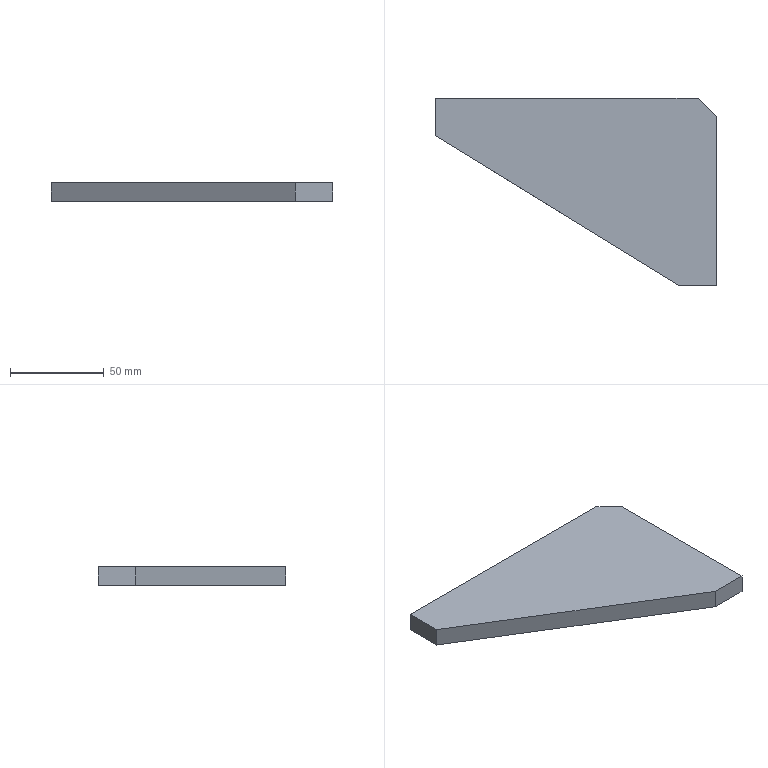Part | SolidWorks | features Chamfer 1, Extrusion 1 | 1 solid | 8 faces | box 150 x 100 x 10 mm | volume 97500 mm3 | plane 8
STEP:
#1=CARTESIAN_POINT('',(-150.,0.,0.));
#2=VERTEX_POINT('',#1);
#3=CARTESIAN_POINT('',(-150.,-20.,0.));
#4=VERTEX_POINT('',#3);
#5=CARTESIAN_POINT('',(-150.,0.,0.));
#6=DIRECTION('',(0.,-1.,0.));
#7=VECTOR('',#6,1000.);
#8=LINE('',#5,#7);
#9=EDGE_CURVE('',#2,#4,#8,.T.);
#10=ORIENTED_EDGE('',*,*,#9,.F.);
#11=CARTESIAN_POINT('',(-150.,0.,-10.));
#12=VERTEX_POINT('',#11);
#13=CARTESIAN_POINT('',(-150.,0.,-10.));
#14=DIRECTION('',(0.,0.,1.));
#15=VECTOR('',#14,1000.);
#16=LINE('',#13,#15);
#17=EDGE_CURVE('',#12,#2,#16,.T.);
#18=ORIENTED_EDGE('',*,*,#17,.F.);
#19=CARTESIAN_POINT('',(-150.,-20.,-10.));
#20=VERTEX_POINT('',#19);
#21=CARTESIAN_POINT('',(-150.,0.,-10.));
#22=DIRECTION('',(0.,-1.,0.));
#23=VECTOR('',#22,1000.);
#24=LINE('',#21,#23);
#25=EDGE_CURVE('',#12,#20,#24,.T.);
#26=ORIENTED_EDGE('',*,*,#25,.T.);
#27=CARTESIAN_POINT('',(-150.,-20.,-10.));
#28=DIRECTION('',(0.,0.,1.));
#29=VECTOR('',#28,1000.);
#30=LINE('',#27,#29);
#31=EDGE_CURVE('',#20,#4,#30,.T.);
#32=ORIENTED_EDGE('',*,*,#31,.T.);
#33=EDGE_LOOP('',(#10,#18,#26,#32));
#34=FACE_OUTER_BOUND('',#33,.T.);
#35=CARTESIAN_POINT('',(-150.,0.,-10.));
#36=DIRECTION('',(-1.,0.,0.));
#37=DIRECTION('',(0.,0.,1.));
#38=AXIS2_PLACEMENT_3D('',#35,#36,#37);
#39=PLANE('',#38);
#40=ADVANCED_FACE('',(#34),#39,.T.);
#41=CARTESIAN_POINT('',(-10.,0.,0.));
#42=VERTEX_POINT('',#41);
#43=CARTESIAN_POINT('',(0.,0.,0.));
#44=DIRECTION('',(-1.,0.,0.));
#45=VECTOR('',#44,1000.);
#46=LINE('',#43,#45);
#47=EDGE_CURVE('',#42,#2,#46,.T.);
#48=ORIENTED_EDGE('',*,*,#47,.F.);
#49=CARTESIAN_POINT('',(-10.,0.,-10.));
#50=VERTEX_POINT('',#49);
#51=CARTESIAN_POINT('',(-10.,0.,-10.));
#52=DIRECTION('',(0.,0.,-1.));
#53=VECTOR('',#52,1000.);
#54=LINE('',#51,#53);
#55=EDGE_CURVE('',#42,#50,#54,.T.);
#56=ORIENTED_EDGE('',*,*,#55,.T.);
#57=CARTESIAN_POINT('',(0.,0.,-10.));
#58=DIRECTION('',(-1.,0.,0.));
#59=VECTOR('',#58,1000.);
#60=LINE('',#57,#59);
#61=EDGE_CURVE('',#50,#12,#60,.T.);
#62=ORIENTED_EDGE('',*,*,#61,.T.);
#63=ORIENTED_EDGE('',*,*,#17,.T.);
#64=EDGE_LOOP('',(#48,#56,#62,#63));
#65=FACE_OUTER_BOUND('',#64,.T.);
#66=CARTESIAN_POINT('',(0.,0.,-10.));
#67=DIRECTION('',(0.,1.,0.));
#68=DIRECTION('',(-1.,0.,0.));
#69=AXIS2_PLACEMENT_3D('',#66,#67,#68);
#70=PLANE('',#69);
#71=ADVANCED_FACE('',(#65),#70,.T.);
#72=CARTESIAN_POINT('',(0.,-100.,-10.));
#73=VERTEX_POINT('',#72);
#74=CARTESIAN_POINT('',(0.,-10.,-10.));
#75=VERTEX_POINT('',#74);
#76=CARTESIAN_POINT('',(0.,-100.,-10.));
#77=DIRECTION('',(0.,1.,0.));
#78=VECTOR('',#77,1000.);
#79=LINE('',#76,#78);
#80=EDGE_CURVE('',#73,#75,#79,.T.);
#81=ORIENTED_EDGE('',*,*,#80,.T.);
#82=CARTESIAN_POINT('',(0.,-10.,0.));
#83=VERTEX_POINT('',#82);
#84=CARTESIAN_POINT('',(0.,-10.,-10.));
#85=DIRECTION('',(0.,0.,1.));
#86=VECTOR('',#85,1000.);
#87=LINE('',#84,#86);
#88=EDGE_CURVE('',#75,#83,#87,.T.);
#89=ORIENTED_EDGE('',*,*,#88,.T.);
#90=CARTESIAN_POINT('',(0.,-100.,0.));
#91=VERTEX_POINT('',#90);
#92=CARTESIAN_POINT('',(0.,-100.,0.));
#93=DIRECTION('',(0.,1.,0.));
#94=VECTOR('',#93,1000.);
#95=LINE('',#92,#94);
#96=EDGE_CURVE('',#91,#83,#95,.T.);
#97=ORIENTED_EDGE('',*,*,#96,.F.);
#98=CARTESIAN_POINT('',(0.,-100.,-10.));
#99=DIRECTION('',(0.,0.,1.));
#100=VECTOR('',#99,1000.);
#101=LINE('',#98,#100);
#102=EDGE_CURVE('',#73,#91,#101,.T.);
#103=ORIENTED_EDGE('',*,*,#102,.F.);
#104=EDGE_LOOP('',(#81,#89,#97,#103));
#105=FACE_OUTER_BOUND('',#104,.T.);
#106=CARTESIAN_POINT('',(0.,-100.,-10.));
#107=DIRECTION('',(1.,0.,0.));
#108=DIRECTION('',(0.,0.,-1.));
#109=AXIS2_PLACEMENT_3D('',#106,#107,#108);
#110=PLANE('',#109);
#111=ADVANCED_FACE('',(#105),#110,.T.);
#112=CARTESIAN_POINT('',(-20.,-100.,0.));
#113=VERTEX_POINT('',#112);
#114=CARTESIAN_POINT('',(-20.,-100.,0.));
#115=DIRECTION('',(1.,0.,0.));
#116=VECTOR('',#115,1000.);
#117=LINE('',#114,#116);
#118=EDGE_CURVE('',#113,#91,#117,.T.);
#119=ORIENTED_EDGE('',*,*,#118,.F.);
#120=CARTESIAN_POINT('',(-20.,-100.,-10.));
#121=VERTEX_POINT('',#120);
#122=CARTESIAN_POINT('',(-20.,-100.,-10.));
#123=DIRECTION('',(0.,0.,1.));
#124=VECTOR('',#123,1000.);
#125=LINE('',#122,#124);
#126=EDGE_CURVE('',#121,#113,#125,.T.);
#127=ORIENTED_EDGE('',*,*,#126,.F.);
#128=CARTESIAN_POINT('',(-20.,-100.,-10.));
#129=DIRECTION('',(1.,0.,0.));
#130=VECTOR('',#129,1000.);
#131=LINE('',#128,#130);
#132=EDGE_CURVE('',#121,#73,#131,.T.);
#133=ORIENTED_EDGE('',*,*,#132,.T.);
#134=ORIENTED_EDGE('',*,*,#102,.T.);
#135=EDGE_LOOP('',(#119,#127,#133,#134));
#136=FACE_OUTER_BOUND('',#135,.T.);
#137=CARTESIAN_POINT('',(-20.,-100.,-10.));
#138=DIRECTION('',(0.,-1.,0.));
#139=DIRECTION('',(0.,0.,-1.));
#140=AXIS2_PLACEMENT_3D('',#137,#138,#139);
#141=PLANE('',#140);
#142=ADVANCED_FACE('',(#136),#141,.T.);
#143=CARTESIAN_POINT('',(-150.,-20.,0.));
#144=DIRECTION('',(0.8517,-0.5241,0.));
#145=VECTOR('',#144,1000.);
#146=LINE('',#143,#145);
#147=EDGE_CURVE('',#4,#113,#146,.T.);
#148=ORIENTED_EDGE('',*,*,#147,.F.);
#149=ORIENTED_EDGE('',*,*,#31,.F.);
#150=CARTESIAN_POINT('',(-150.,-20.,-10.));
#151=DIRECTION('',(0.8517,-0.5241,0.));
#152=VECTOR('',#151,1000.);
#153=LINE('',#150,#152);
#154=EDGE_CURVE('',#20,#121,#153,.T.);
#155=ORIENTED_EDGE('',*,*,#154,.T.);
#156=ORIENTED_EDGE('',*,*,#126,.T.);
#157=EDGE_LOOP('',(#148,#149,#155,#156));
#158=FACE_OUTER_BOUND('',#157,.T.);
#159=CARTESIAN_POINT('',(-150.,-20.,-10.));
#160=DIRECTION('',(-0.5241,-0.8517,0.));
#161=DIRECTION('',(0.8517,-0.5241,0.));
#162=AXIS2_PLACEMENT_3D('',#159,#160,#161);
#163=PLANE('',#162);
#164=ADVANCED_FACE('',(#158),#163,.T.);
#165=ORIENTED_EDGE('',*,*,#61,.F.);
#166=CARTESIAN_POINT('',(0.,-10.,-10.));
#167=DIRECTION('',(0.7071,-0.7071,0.));
#168=VECTOR('',#167,1000.);
#169=LINE('',#166,#168);
#170=EDGE_CURVE('',#50,#75,#169,.T.);
#171=ORIENTED_EDGE('',*,*,#170,.T.);
#172=ORIENTED_EDGE('',*,*,#80,.F.);
#173=ORIENTED_EDGE('',*,*,#132,.F.);
#174=ORIENTED_EDGE('',*,*,#154,.F.);
#175=ORIENTED_EDGE('',*,*,#25,.F.);
#176=EDGE_LOOP('',(#165,#171,#172,#173,#174,#175));
#177=FACE_OUTER_BOUND('',#176,.T.);
#178=CARTESIAN_POINT('',(0.,0.,-10.));
#179=DIRECTION('',(0.,0.,1.));
#180=DIRECTION('',(1.,0.,0.));
#181=AXIS2_PLACEMENT_3D('',#178,#179,#180);
#182=PLANE('',#181);
#183=ADVANCED_FACE('',(#177),#182,.F.);
#184=ORIENTED_EDGE('',*,*,#96,.T.);
#185=CARTESIAN_POINT('',(-5.,-5.,0.));
#186=DIRECTION('',(-0.7071,0.7071,0.));
#187=VECTOR('',#186,1000.);
#188=LINE('',#185,#187);
#189=EDGE_CURVE('',#83,#42,#188,.T.);
#190=ORIENTED_EDGE('',*,*,#189,.T.);
#191=ORIENTED_EDGE('',*,*,#47,.T.);
#192=ORIENTED_EDGE('',*,*,#9,.T.);
#193=ORIENTED_EDGE('',*,*,#147,.T.);
#194=ORIENTED_EDGE('',*,*,#118,.T.);
#195=EDGE_LOOP('',(#184,#190,#191,#192,#193,#194));
#196=FACE_OUTER_BOUND('',#195,.T.);
#197=CARTESIAN_POINT('',(0.,0.,0.));
#198=DIRECTION('',(0.,0.,1.));
#199=DIRECTION('',(1.,0.,0.));
#200=AXIS2_PLACEMENT_3D('',#197,#198,#199);
#201=PLANE('',#200);
#202=ADVANCED_FACE('',(#196),#201,.T.);
#203=ORIENTED_EDGE('',*,*,#170,.F.);
#204=ORIENTED_EDGE('',*,*,#55,.F.);
#205=ORIENTED_EDGE('',*,*,#189,.F.);
#206=ORIENTED_EDGE('',*,*,#88,.F.);
#207=EDGE_LOOP('',(#203,#204,#205,#206));
#208=FACE_OUTER_BOUND('',#207,.T.);
#209=CARTESIAN_POINT('',(0.,-10.,-10.));
#210=DIRECTION('',(-0.7071,-0.7071,0.));
#211=DIRECTION('',(0.,0.,1.));
#212=AXIS2_PLACEMENT_3D('',#209,#210,#211);
#213=PLANE('',#212);
#214=ADVANCED_FACE('',(#208),#213,.F.);
#215=CLOSED_SHELL('',(#40,#71,#111,#142,#164,#183,#202,#214));
#216=MANIFOLD_SOLID_BREP('',#215);
#217=CARTESIAN_POINT('',(0.,0.,0.));
#218=DIRECTION('',(0.,0.,1.));
#219=DIRECTION('',(1.,0.,0.));
#220=AXIS2_PLACEMENT_3D('',#217,#218,#219);
#221=(LENGTH_UNIT()NAMED_UNIT(*)SI_UNIT(.MILLI.,.METRE.));
#222=UNCERTAINTY_MEASURE_WITH_UNIT(LENGTH_MEASURE(0.00001),#221,'','');
#223=(NAMED_UNIT(*)PLANE_ANGLE_UNIT()SI_UNIT($,.RADIAN.));
#224=(NAMED_UNIT(*)SI_UNIT($,.STERADIAN.)SOLID_ANGLE_UNIT());
#225=(GEOMETRIC_REPRESENTATION_CONTEXT(3)GLOBAL_UNCERTAINTY_ASSIGNED_CONTEXT((#222))GLOBAL_UNIT_ASSIGNED_CONTEXT((#221,#223,#224))REPRESENTATION_CONTEXT('',''));
#226=ADVANCED_BREP_SHAPE_REPRESENTATION('',(#216,#220),#225);